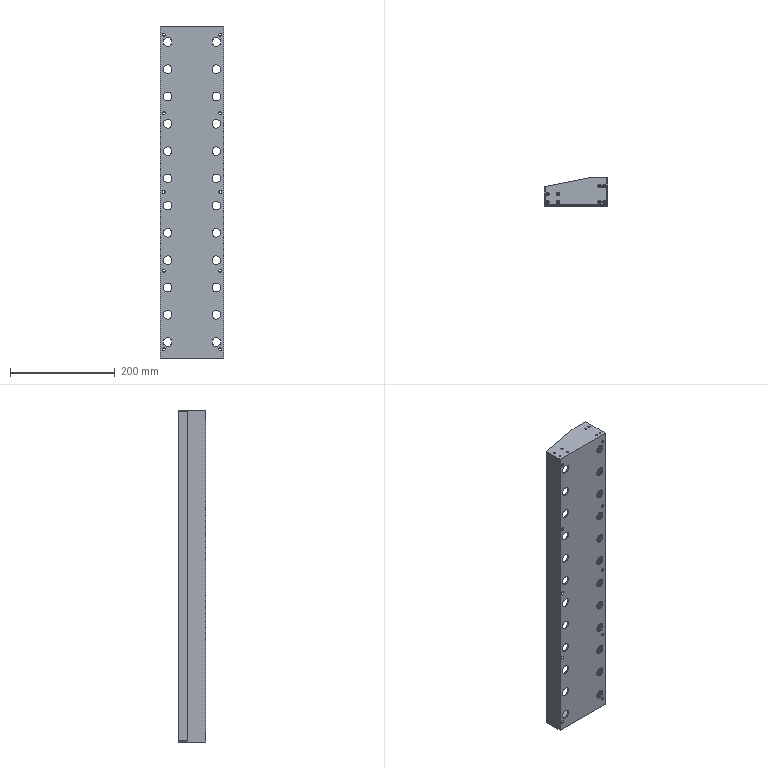Part | STEP file | Storage box shell | 1 solid | 146 faces | box 122 x 53 x 633 mm | volume 271633 mm3 | cylinder 80 | cone 52 | plane 14 | commonest cylinder face diameters 16.5 x48 3.4 x32